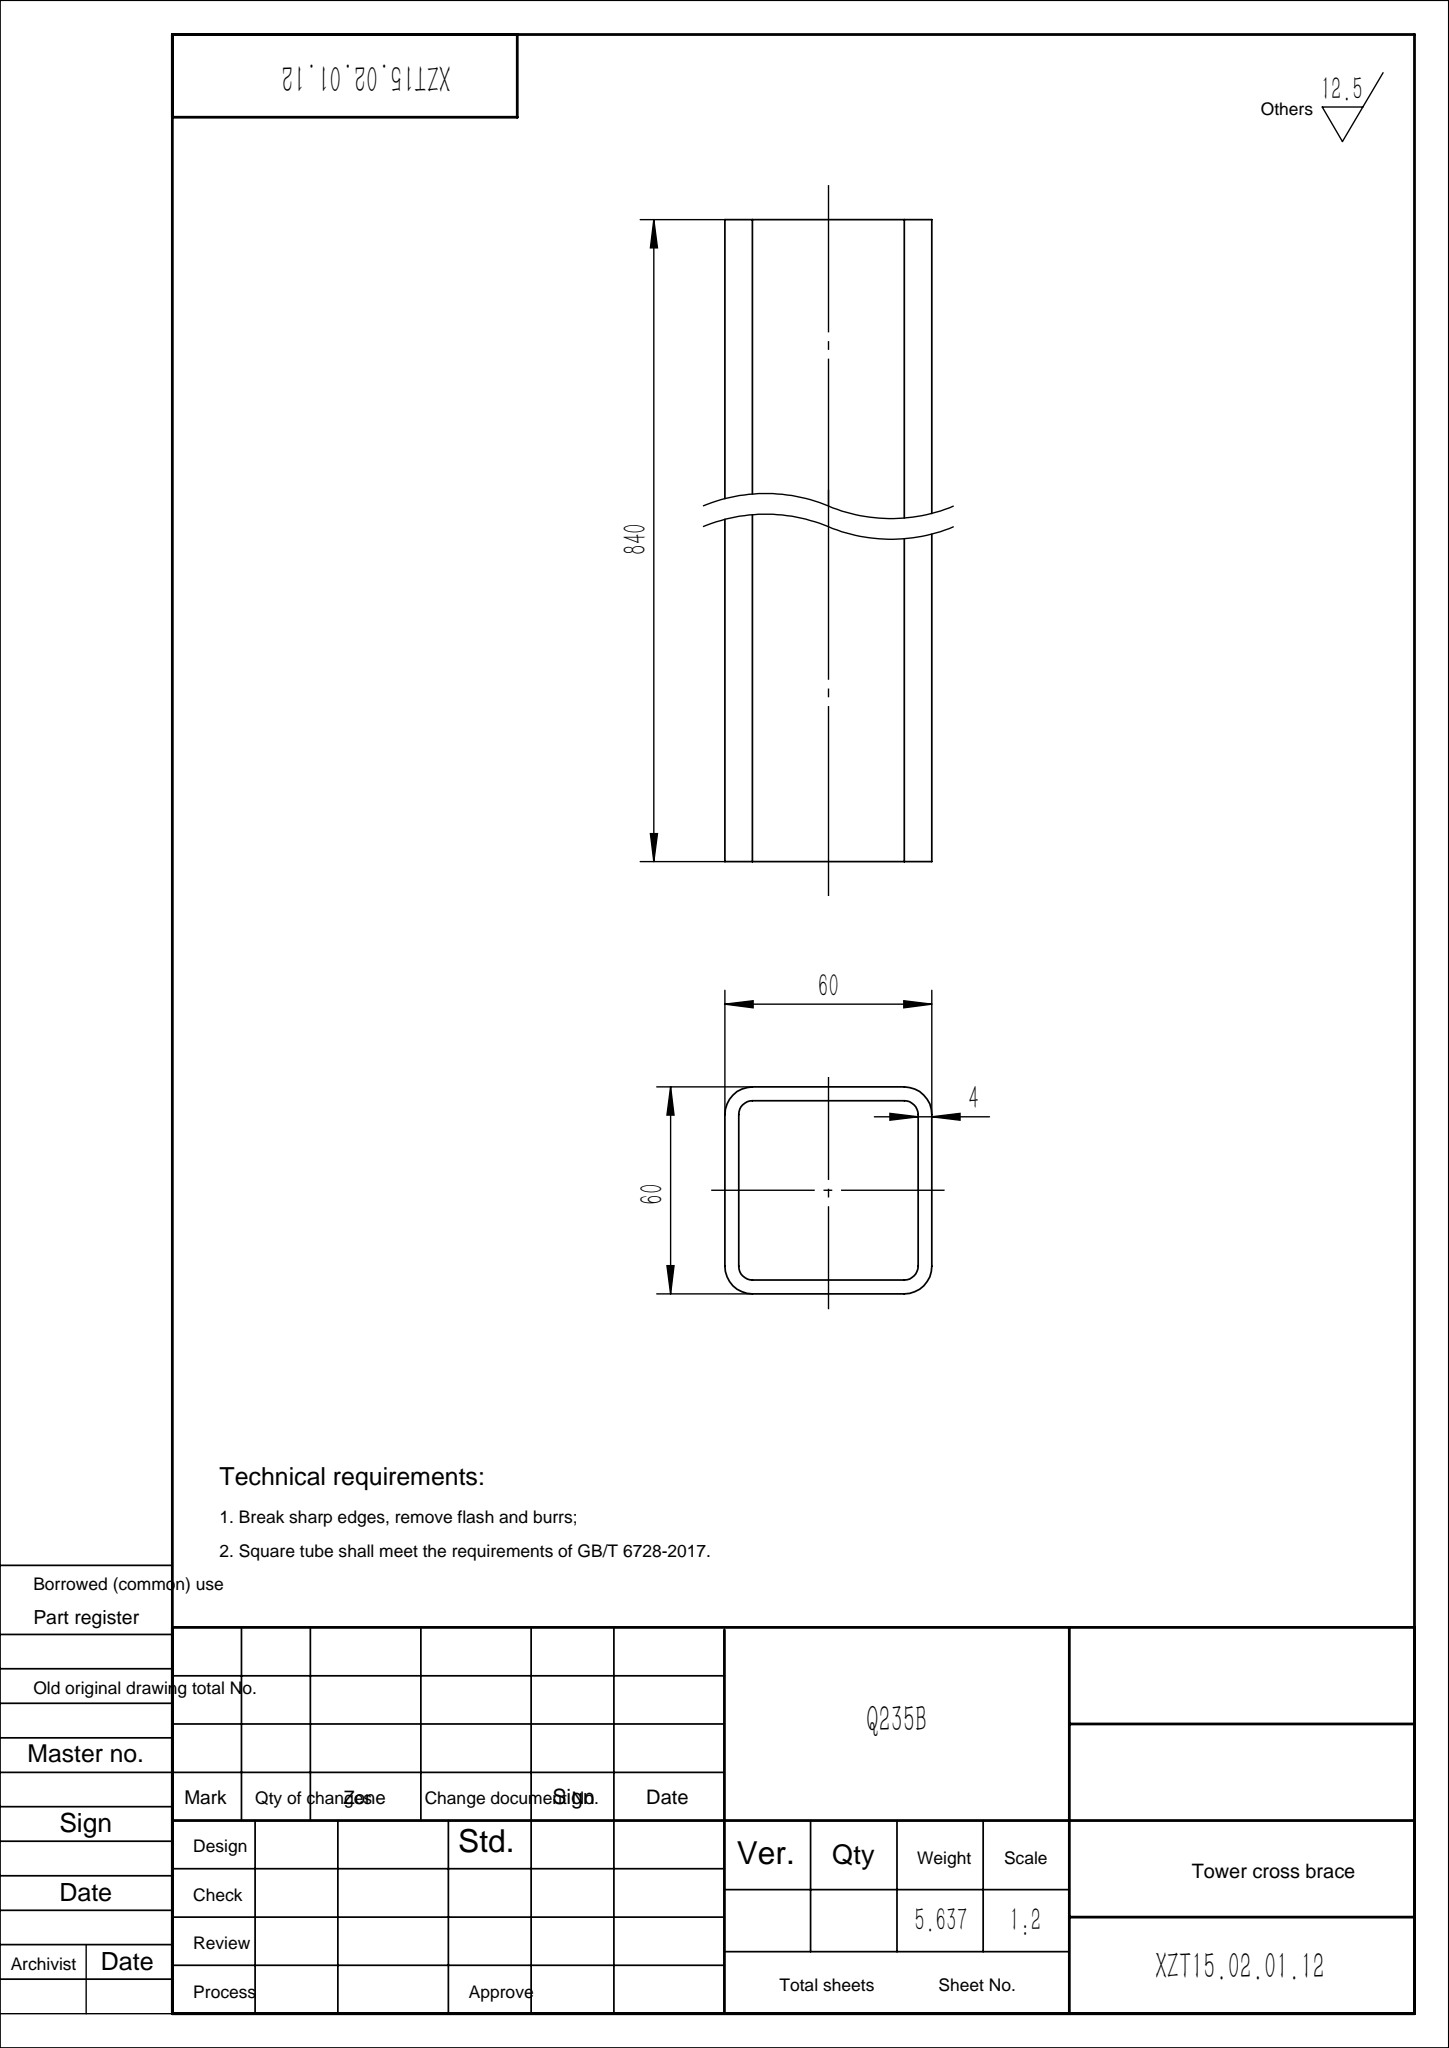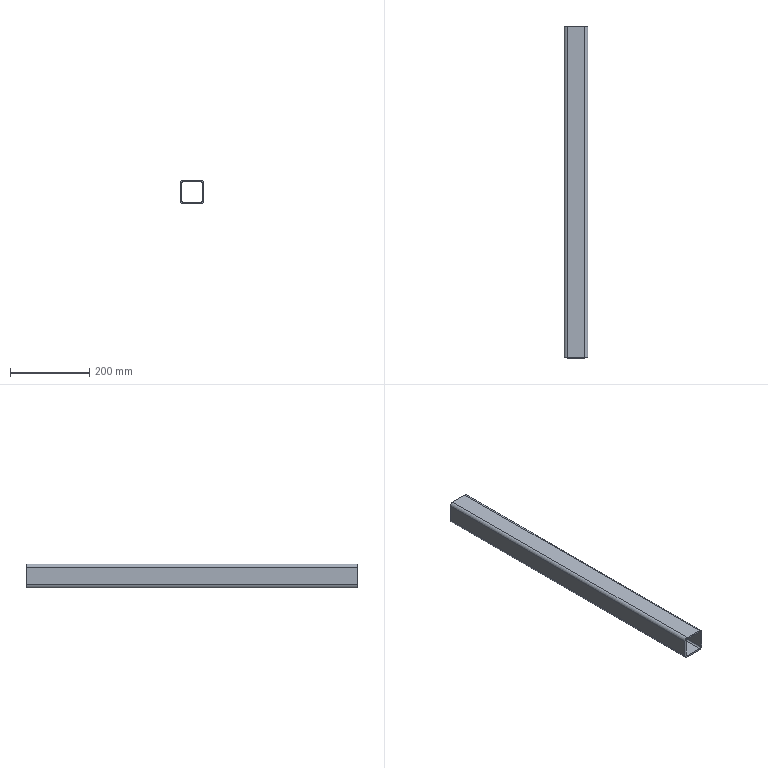Part | SolidWorks | features WeldMemberFeat 1, WeldmentFeature 1 | 1 solid | 18 faces | box 60 x 840 x 60 mm | volume 718029 mm3 | plane 10 | cylinder 8 | commonest cylinder face diameters 8 x4 16 x4
STEP:
#1=CARTESIAN_POINT('',(-30.,0.,22.));
#2=VERTEX_POINT('',#1);
#3=CARTESIAN_POINT('',(-22.,0.,30.));
#4=VERTEX_POINT('',#3);
#5=CARTESIAN_POINT('',(-22.,0.,22.));
#6=DIRECTION('',(0.,1.,0.));
#7=DIRECTION('',(0.,0.,1.));
#8=AXIS2_PLACEMENT_3D('',#5,#6,#7);
#9=CIRCLE('',#8,8.);
#10=EDGE_CURVE('',#2,#4,#9,.T.);
#11=ORIENTED_EDGE('',*,*,#10,.T.);
#12=CARTESIAN_POINT('',(-22.,840.,30.));
#13=VERTEX_POINT('',#12);
#14=CARTESIAN_POINT('',(-22.,840.,30.));
#15=DIRECTION('',(0.,-1.,0.));
#16=VECTOR('',#15,1000.);
#17=LINE('',#14,#16);
#18=EDGE_CURVE('',#13,#4,#17,.T.);
#19=ORIENTED_EDGE('',*,*,#18,.F.);
#20=CARTESIAN_POINT('',(-30.,840.,22.));
#21=VERTEX_POINT('',#20);
#22=CARTESIAN_POINT('',(-22.,840.,22.));
#23=DIRECTION('',(0.,1.,0.));
#24=DIRECTION('',(0.,0.,1.));
#25=AXIS2_PLACEMENT_3D('',#22,#23,#24);
#26=CIRCLE('',#25,8.);
#27=EDGE_CURVE('',#21,#13,#26,.T.);
#28=ORIENTED_EDGE('',*,*,#27,.F.);
#29=CARTESIAN_POINT('',(-30.,840.,22.));
#30=DIRECTION('',(0.,-1.,0.));
#31=VECTOR('',#30,1000.);
#32=LINE('',#29,#31);
#33=EDGE_CURVE('',#21,#2,#32,.T.);
#34=ORIENTED_EDGE('',*,*,#33,.T.);
#35=EDGE_LOOP('',(#11,#19,#28,#34));
#36=FACE_OUTER_BOUND('',#35,.T.);
#37=CARTESIAN_POINT('',(-22.,840.,22.));
#38=DIRECTION('',(0.,-1.,0.));
#39=DIRECTION('',(0.,0.,-1.));
#40=AXIS2_PLACEMENT_3D('',#37,#38,#39);
#41=CYLINDRICAL_SURFACE('',#40,8.);
#42=ADVANCED_FACE('',(#36),#41,.T.);
#43=CARTESIAN_POINT('',(22.,0.,30.));
#44=VERTEX_POINT('',#43);
#45=CARTESIAN_POINT('',(-22.,0.,30.));
#46=DIRECTION('',(1.,0.,0.));
#47=VECTOR('',#46,1000.);
#48=LINE('',#45,#47);
#49=EDGE_CURVE('',#4,#44,#48,.T.);
#50=ORIENTED_EDGE('',*,*,#49,.T.);
#51=CARTESIAN_POINT('',(22.,840.,30.));
#52=VERTEX_POINT('',#51);
#53=CARTESIAN_POINT('',(22.,840.,30.));
#54=DIRECTION('',(0.,-1.,0.));
#55=VECTOR('',#54,1000.);
#56=LINE('',#53,#55);
#57=EDGE_CURVE('',#52,#44,#56,.T.);
#58=ORIENTED_EDGE('',*,*,#57,.F.);
#59=CARTESIAN_POINT('',(-22.,840.,30.));
#60=DIRECTION('',(1.,0.,0.));
#61=VECTOR('',#60,1000.);
#62=LINE('',#59,#61);
#63=EDGE_CURVE('',#13,#52,#62,.T.);
#64=ORIENTED_EDGE('',*,*,#63,.F.);
#65=ORIENTED_EDGE('',*,*,#18,.T.);
#66=EDGE_LOOP('',(#50,#58,#64,#65));
#67=FACE_OUTER_BOUND('',#66,.T.);
#68=CARTESIAN_POINT('',(-22.,840.,30.));
#69=DIRECTION('',(0.,0.,-1.));
#70=DIRECTION('',(-1.,0.,0.));
#71=AXIS2_PLACEMENT_3D('',#68,#69,#70);
#72=PLANE('',#71);
#73=ADVANCED_FACE('',(#67),#72,.F.);
#74=CARTESIAN_POINT('',(30.,0.,22.));
#75=VERTEX_POINT('',#74);
#76=CARTESIAN_POINT('',(22.,0.,22.));
#77=DIRECTION('',(0.,1.,0.));
#78=DIRECTION('',(0.,0.,1.));
#79=AXIS2_PLACEMENT_3D('',#76,#77,#78);
#80=CIRCLE('',#79,8.);
#81=EDGE_CURVE('',#44,#75,#80,.T.);
#82=ORIENTED_EDGE('',*,*,#81,.T.);
#83=CARTESIAN_POINT('',(30.,840.,22.));
#84=VERTEX_POINT('',#83);
#85=CARTESIAN_POINT('',(30.,840.,22.));
#86=DIRECTION('',(0.,-1.,0.));
#87=VECTOR('',#86,1000.);
#88=LINE('',#85,#87);
#89=EDGE_CURVE('',#84,#75,#88,.T.);
#90=ORIENTED_EDGE('',*,*,#89,.F.);
#91=CARTESIAN_POINT('',(22.,840.,22.));
#92=DIRECTION('',(0.,1.,0.));
#93=DIRECTION('',(0.,0.,1.));
#94=AXIS2_PLACEMENT_3D('',#91,#92,#93);
#95=CIRCLE('',#94,8.);
#96=EDGE_CURVE('',#52,#84,#95,.T.);
#97=ORIENTED_EDGE('',*,*,#96,.F.);
#98=ORIENTED_EDGE('',*,*,#57,.T.);
#99=EDGE_LOOP('',(#82,#90,#97,#98));
#100=FACE_OUTER_BOUND('',#99,.T.);
#101=CARTESIAN_POINT('',(22.,840.,22.));
#102=DIRECTION('',(0.,-1.,0.));
#103=DIRECTION('',(0.,0.,-1.));
#104=AXIS2_PLACEMENT_3D('',#101,#102,#103);
#105=CYLINDRICAL_SURFACE('',#104,8.);
#106=ADVANCED_FACE('',(#100),#105,.T.);
#107=CARTESIAN_POINT('',(30.,0.,-22.));
#108=VERTEX_POINT('',#107);
#109=CARTESIAN_POINT('',(30.,0.,-22.));
#110=DIRECTION('',(0.,0.,-1.));
#111=VECTOR('',#110,1000.);
#112=LINE('',#109,#111);
#113=EDGE_CURVE('',#75,#108,#112,.T.);
#114=ORIENTED_EDGE('',*,*,#113,.T.);
#115=CARTESIAN_POINT('',(30.,840.,-22.));
#116=VERTEX_POINT('',#115);
#117=CARTESIAN_POINT('',(30.,840.,-22.));
#118=DIRECTION('',(0.,-1.,0.));
#119=VECTOR('',#118,1000.);
#120=LINE('',#117,#119);
#121=EDGE_CURVE('',#116,#108,#120,.T.);
#122=ORIENTED_EDGE('',*,*,#121,.F.);
#123=CARTESIAN_POINT('',(30.,840.,-22.));
#124=DIRECTION('',(0.,0.,-1.));
#125=VECTOR('',#124,1000.);
#126=LINE('',#123,#125);
#127=EDGE_CURVE('',#84,#116,#126,.T.);
#128=ORIENTED_EDGE('',*,*,#127,.F.);
#129=ORIENTED_EDGE('',*,*,#89,.T.);
#130=EDGE_LOOP('',(#114,#122,#128,#129));
#131=FACE_OUTER_BOUND('',#130,.T.);
#132=CARTESIAN_POINT('',(30.,840.,-22.));
#133=DIRECTION('',(-1.,0.,0.));
#134=DIRECTION('',(0.,0.,1.));
#135=AXIS2_PLACEMENT_3D('',#132,#133,#134);
#136=PLANE('',#135);
#137=ADVANCED_FACE('',(#131),#136,.F.);
#138=CARTESIAN_POINT('',(22.,0.,-30.));
#139=VERTEX_POINT('',#138);
#140=CARTESIAN_POINT('',(22.,0.,-22.));
#141=DIRECTION('',(0.,1.,0.));
#142=DIRECTION('',(0.,0.,1.));
#143=AXIS2_PLACEMENT_3D('',#140,#141,#142);
#144=CIRCLE('',#143,8.);
#145=EDGE_CURVE('',#108,#139,#144,.T.);
#146=ORIENTED_EDGE('',*,*,#145,.T.);
#147=CARTESIAN_POINT('',(22.,840.,-30.));
#148=VERTEX_POINT('',#147);
#149=CARTESIAN_POINT('',(22.,840.,-30.));
#150=DIRECTION('',(0.,-1.,0.));
#151=VECTOR('',#150,1000.);
#152=LINE('',#149,#151);
#153=EDGE_CURVE('',#148,#139,#152,.T.);
#154=ORIENTED_EDGE('',*,*,#153,.F.);
#155=CARTESIAN_POINT('',(22.,840.,-22.));
#156=DIRECTION('',(0.,1.,0.));
#157=DIRECTION('',(0.,0.,1.));
#158=AXIS2_PLACEMENT_3D('',#155,#156,#157);
#159=CIRCLE('',#158,8.);
#160=EDGE_CURVE('',#116,#148,#159,.T.);
#161=ORIENTED_EDGE('',*,*,#160,.F.);
#162=ORIENTED_EDGE('',*,*,#121,.T.);
#163=EDGE_LOOP('',(#146,#154,#161,#162));
#164=FACE_OUTER_BOUND('',#163,.T.);
#165=CARTESIAN_POINT('',(22.,840.,-22.));
#166=DIRECTION('',(0.,-1.,0.));
#167=DIRECTION('',(0.,0.,-1.));
#168=AXIS2_PLACEMENT_3D('',#165,#166,#167);
#169=CYLINDRICAL_SURFACE('',#168,8.);
#170=ADVANCED_FACE('',(#164),#169,.T.);
#171=CARTESIAN_POINT('',(-22.,0.,-30.));
#172=VERTEX_POINT('',#171);
#173=CARTESIAN_POINT('',(22.,0.,-30.));
#174=DIRECTION('',(-1.,0.,0.));
#175=VECTOR('',#174,1000.);
#176=LINE('',#173,#175);
#177=EDGE_CURVE('',#139,#172,#176,.T.);
#178=ORIENTED_EDGE('',*,*,#177,.T.);
#179=CARTESIAN_POINT('',(-22.,840.,-30.));
#180=VERTEX_POINT('',#179);
#181=CARTESIAN_POINT('',(-22.,840.,-30.));
#182=DIRECTION('',(0.,-1.,0.));
#183=VECTOR('',#182,1000.);
#184=LINE('',#181,#183);
#185=EDGE_CURVE('',#180,#172,#184,.T.);
#186=ORIENTED_EDGE('',*,*,#185,.F.);
#187=CARTESIAN_POINT('',(22.,840.,-30.));
#188=DIRECTION('',(-1.,0.,0.));
#189=VECTOR('',#188,1000.);
#190=LINE('',#187,#189);
#191=EDGE_CURVE('',#148,#180,#190,.T.);
#192=ORIENTED_EDGE('',*,*,#191,.F.);
#193=ORIENTED_EDGE('',*,*,#153,.T.);
#194=EDGE_LOOP('',(#178,#186,#192,#193));
#195=FACE_OUTER_BOUND('',#194,.T.);
#196=CARTESIAN_POINT('',(22.,840.,-30.));
#197=DIRECTION('',(0.,0.,1.));
#198=DIRECTION('',(1.,0.,0.));
#199=AXIS2_PLACEMENT_3D('',#196,#197,#198);
#200=PLANE('',#199);
#201=ADVANCED_FACE('',(#195),#200,.F.);
#202=CARTESIAN_POINT('',(-30.,0.,-22.));
#203=VERTEX_POINT('',#202);
#204=CARTESIAN_POINT('',(-22.,0.,-22.));
#205=DIRECTION('',(0.,1.,0.));
#206=DIRECTION('',(0.,0.,1.));
#207=AXIS2_PLACEMENT_3D('',#204,#205,#206);
#208=CIRCLE('',#207,8.);
#209=EDGE_CURVE('',#172,#203,#208,.T.);
#210=ORIENTED_EDGE('',*,*,#209,.T.);
#211=CARTESIAN_POINT('',(-30.,840.,-22.));
#212=VERTEX_POINT('',#211);
#213=CARTESIAN_POINT('',(-30.,840.,-22.));
#214=DIRECTION('',(0.,-1.,0.));
#215=VECTOR('',#214,1000.);
#216=LINE('',#213,#215);
#217=EDGE_CURVE('',#212,#203,#216,.T.);
#218=ORIENTED_EDGE('',*,*,#217,.F.);
#219=CARTESIAN_POINT('',(-22.,840.,-22.));
#220=DIRECTION('',(0.,1.,0.));
#221=DIRECTION('',(0.,0.,1.));
#222=AXIS2_PLACEMENT_3D('',#219,#220,#221);
#223=CIRCLE('',#222,8.);
#224=EDGE_CURVE('',#180,#212,#223,.T.);
#225=ORIENTED_EDGE('',*,*,#224,.F.);
#226=ORIENTED_EDGE('',*,*,#185,.T.);
#227=EDGE_LOOP('',(#210,#218,#225,#226));
#228=FACE_OUTER_BOUND('',#227,.T.);
#229=CARTESIAN_POINT('',(-22.,840.,-22.));
#230=DIRECTION('',(0.,-1.,0.));
#231=DIRECTION('',(0.,0.,-1.));
#232=AXIS2_PLACEMENT_3D('',#229,#230,#231);
#233=CYLINDRICAL_SURFACE('',#232,8.);
#234=ADVANCED_FACE('',(#228),#233,.T.);
#235=CARTESIAN_POINT('',(22.,0.,26.));
#236=VERTEX_POINT('',#235);
#237=CARTESIAN_POINT('',(26.,0.,22.));
#238=VERTEX_POINT('',#237);
#239=CARTESIAN_POINT('',(22.,0.,22.));
#240=DIRECTION('',(0.,1.,0.));
#241=DIRECTION('',(0.,0.,1.));
#242=AXIS2_PLACEMENT_3D('',#239,#240,#241);
#243=CIRCLE('',#242,4.);
#244=EDGE_CURVE('',#236,#238,#243,.T.);
#245=ORIENTED_EDGE('',*,*,#244,.F.);
#246=CARTESIAN_POINT('',(22.,840.,26.));
#247=VERTEX_POINT('',#246);
#248=CARTESIAN_POINT('',(22.,840.,26.));
#249=DIRECTION('',(0.,-1.,0.));
#250=VECTOR('',#249,1000.);
#251=LINE('',#248,#250);
#252=EDGE_CURVE('',#247,#236,#251,.T.);
#253=ORIENTED_EDGE('',*,*,#252,.F.);
#254=CARTESIAN_POINT('',(26.,840.,22.));
#255=VERTEX_POINT('',#254);
#256=CARTESIAN_POINT('',(22.,840.,22.));
#257=DIRECTION('',(0.,1.,0.));
#258=DIRECTION('',(0.,0.,1.));
#259=AXIS2_PLACEMENT_3D('',#256,#257,#258);
#260=CIRCLE('',#259,4.);
#261=EDGE_CURVE('',#247,#255,#260,.T.);
#262=ORIENTED_EDGE('',*,*,#261,.T.);
#263=CARTESIAN_POINT('',(26.,840.,22.));
#264=DIRECTION('',(0.,-1.,0.));
#265=VECTOR('',#264,1000.);
#266=LINE('',#263,#265);
#267=EDGE_CURVE('',#255,#238,#266,.T.);
#268=ORIENTED_EDGE('',*,*,#267,.T.);
#269=EDGE_LOOP('',(#245,#253,#262,#268));
#270=FACE_OUTER_BOUND('',#269,.T.);
#271=CARTESIAN_POINT('',(22.,840.,22.));
#272=DIRECTION('',(0.,-1.,0.));
#273=DIRECTION('',(0.,0.,-1.));
#274=AXIS2_PLACEMENT_3D('',#271,#272,#273);
#275=CYLINDRICAL_SURFACE('',#274,4.);
#276=ADVANCED_FACE('',(#270),#275,.F.);
#277=CARTESIAN_POINT('',(-22.,0.,26.));
#278=VERTEX_POINT('',#277);
#279=CARTESIAN_POINT('',(-22.,0.,26.));
#280=DIRECTION('',(1.,0.,0.));
#281=VECTOR('',#280,1000.);
#282=LINE('',#279,#281);
#283=EDGE_CURVE('',#278,#236,#282,.T.);
#284=ORIENTED_EDGE('',*,*,#283,.F.);
#285=CARTESIAN_POINT('',(-22.,840.,26.));
#286=VERTEX_POINT('',#285);
#287=CARTESIAN_POINT('',(-22.,840.,26.));
#288=DIRECTION('',(0.,-1.,0.));
#289=VECTOR('',#288,1000.);
#290=LINE('',#287,#289);
#291=EDGE_CURVE('',#286,#278,#290,.T.);
#292=ORIENTED_EDGE('',*,*,#291,.F.);
#293=CARTESIAN_POINT('',(-22.,840.,26.));
#294=DIRECTION('',(1.,0.,0.));
#295=VECTOR('',#294,1000.);
#296=LINE('',#293,#295);
#297=EDGE_CURVE('',#286,#247,#296,.T.);
#298=ORIENTED_EDGE('',*,*,#297,.T.);
#299=ORIENTED_EDGE('',*,*,#252,.T.);
#300=EDGE_LOOP('',(#284,#292,#298,#299));
#301=FACE_OUTER_BOUND('',#300,.T.);
#302=CARTESIAN_POINT('',(-22.,840.,26.));
#303=DIRECTION('',(0.,0.,-1.));
#304=DIRECTION('',(-1.,0.,0.));
#305=AXIS2_PLACEMENT_3D('',#302,#303,#304);
#306=PLANE('',#305);
#307=ADVANCED_FACE('',(#301),#306,.T.);
#308=CARTESIAN_POINT('',(-26.,0.,22.));
#309=VERTEX_POINT('',#308);
#310=CARTESIAN_POINT('',(-22.,0.,22.));
#311=DIRECTION('',(0.,1.,0.));
#312=DIRECTION('',(0.,0.,1.));
#313=AXIS2_PLACEMENT_3D('',#310,#311,#312);
#314=CIRCLE('',#313,4.);
#315=EDGE_CURVE('',#309,#278,#314,.T.);
#316=ORIENTED_EDGE('',*,*,#315,.F.);
#317=CARTESIAN_POINT('',(-26.,840.,22.));
#318=VERTEX_POINT('',#317);
#319=CARTESIAN_POINT('',(-26.,840.,22.));
#320=DIRECTION('',(0.,-1.,0.));
#321=VECTOR('',#320,1000.);
#322=LINE('',#319,#321);
#323=EDGE_CURVE('',#318,#309,#322,.T.);
#324=ORIENTED_EDGE('',*,*,#323,.F.);
#325=CARTESIAN_POINT('',(-22.,840.,22.));
#326=DIRECTION('',(0.,1.,0.));
#327=DIRECTION('',(0.,0.,1.));
#328=AXIS2_PLACEMENT_3D('',#325,#326,#327);
#329=CIRCLE('',#328,4.);
#330=EDGE_CURVE('',#318,#286,#329,.T.);
#331=ORIENTED_EDGE('',*,*,#330,.T.);
#332=ORIENTED_EDGE('',*,*,#291,.T.);
#333=EDGE_LOOP('',(#316,#324,#331,#332));
#334=FACE_OUTER_BOUND('',#333,.T.);
#335=CARTESIAN_POINT('',(-22.,840.,22.));
#336=DIRECTION('',(0.,-1.,0.));
#337=DIRECTION('',(0.,0.,-1.));
#338=AXIS2_PLACEMENT_3D('',#335,#336,#337);
#339=CYLINDRICAL_SURFACE('',#338,4.);
#340=ADVANCED_FACE('',(#334),#339,.F.);
#341=CARTESIAN_POINT('',(-26.,0.,-22.));
#342=VERTEX_POINT('',#341);
#343=CARTESIAN_POINT('',(-26.,0.,22.));
#344=DIRECTION('',(0.,0.,1.));
#345=VECTOR('',#344,1000.);
#346=LINE('',#343,#345);
#347=EDGE_CURVE('',#342,#309,#346,.T.);
#348=ORIENTED_EDGE('',*,*,#347,.F.);
#349=CARTESIAN_POINT('',(-26.,840.,-22.));
#350=VERTEX_POINT('',#349);
#351=CARTESIAN_POINT('',(-26.,840.,-22.));
#352=DIRECTION('',(0.,-1.,0.));
#353=VECTOR('',#352,1000.);
#354=LINE('',#351,#353);
#355=EDGE_CURVE('',#350,#342,#354,.T.);
#356=ORIENTED_EDGE('',*,*,#355,.F.);
#357=CARTESIAN_POINT('',(-26.,840.,22.));
#358=DIRECTION('',(0.,0.,1.));
#359=VECTOR('',#358,1000.);
#360=LINE('',#357,#359);
#361=EDGE_CURVE('',#350,#318,#360,.T.);
#362=ORIENTED_EDGE('',*,*,#361,.T.);
#363=ORIENTED_EDGE('',*,*,#323,.T.);
#364=EDGE_LOOP('',(#348,#356,#362,#363));
#365=FACE_OUTER_BOUND('',#364,.T.);
#366=CARTESIAN_POINT('',(-26.,840.,22.));
#367=DIRECTION('',(1.,0.,0.));
#368=DIRECTION('',(0.,0.,-1.));
#369=AXIS2_PLACEMENT_3D('',#366,#367,#368);
#370=PLANE('',#369);
#371=ADVANCED_FACE('',(#365),#370,.T.);
#372=CARTESIAN_POINT('',(-22.,0.,-26.));
#373=VERTEX_POINT('',#372);
#374=CARTESIAN_POINT('',(-22.,0.,-22.));
#375=DIRECTION('',(0.,1.,0.));
#376=DIRECTION('',(0.,0.,1.));
#377=AXIS2_PLACEMENT_3D('',#374,#375,#376);
#378=CIRCLE('',#377,4.);
#379=EDGE_CURVE('',#373,#342,#378,.T.);
#380=ORIENTED_EDGE('',*,*,#379,.F.);
#381=CARTESIAN_POINT('',(-22.,840.,-26.));
#382=VERTEX_POINT('',#381);
#383=CARTESIAN_POINT('',(-22.,840.,-26.));
#384=DIRECTION('',(0.,-1.,0.));
#385=VECTOR('',#384,1000.);
#386=LINE('',#383,#385);
#387=EDGE_CURVE('',#382,#373,#386,.T.);
#388=ORIENTED_EDGE('',*,*,#387,.F.);
#389=CARTESIAN_POINT('',(-22.,840.,-22.));
#390=DIRECTION('',(0.,1.,0.));
#391=DIRECTION('',(0.,0.,1.));
#392=AXIS2_PLACEMENT_3D('',#389,#390,#391);
#393=CIRCLE('',#392,4.);
#394=EDGE_CURVE('',#382,#350,#393,.T.);
#395=ORIENTED_EDGE('',*,*,#394,.T.);
#396=ORIENTED_EDGE('',*,*,#355,.T.);
#397=EDGE_LOOP('',(#380,#388,#395,#396));
#398=FACE_OUTER_BOUND('',#397,.T.);
#399=CARTESIAN_POINT('',(-22.,840.,-22.));
#400=DIRECTION('',(0.,-1.,0.));
#401=DIRECTION('',(0.,0.,-1.));
#402=AXIS2_PLACEMENT_3D('',#399,#400,#401);
#403=CYLINDRICAL_SURFACE('',#402,4.);
#404=ADVANCED_FACE('',(#398),#403,.F.);
#405=CARTESIAN_POINT('',(22.,0.,-26.));
#406=VERTEX_POINT('',#405);
#407=CARTESIAN_POINT('',(22.,0.,-26.));
#408=DIRECTION('',(-1.,0.,0.));
#409=VECTOR('',#408,1000.);
#410=LINE('',#407,#409);
#411=EDGE_CURVE('',#406,#373,#410,.T.);
#412=ORIENTED_EDGE('',*,*,#411,.F.);
#413=CARTESIAN_POINT('',(22.,840.,-26.));
#414=VERTEX_POINT('',#413);
#415=CARTESIAN_POINT('',(22.,840.,-26.));
#416=DIRECTION('',(0.,-1.,0.));
#417=VECTOR('',#416,1000.);
#418=LINE('',#415,#417);
#419=EDGE_CURVE('',#414,#406,#418,.T.);
#420=ORIENTED_EDGE('',*,*,#419,.F.);
#421=CARTESIAN_POINT('',(22.,840.,-26.));
#422=DIRECTION('',(-1.,0.,0.));
#423=VECTOR('',#422,1000.);
#424=LINE('',#421,#423);
#425=EDGE_CURVE('',#414,#382,#424,.T.);
#426=ORIENTED_EDGE('',*,*,#425,.T.);
#427=ORIENTED_EDGE('',*,*,#387,.T.);
#428=EDGE_LOOP('',(#412,#420,#426,#427));
#429=FACE_OUTER_BOUND('',#428,.T.);
#430=CARTESIAN_POINT('',(22.,840.,-26.));
#431=DIRECTION('',(0.,0.,1.));
#432=DIRECTION('',(1.,0.,0.));
#433=AXIS2_PLACEMENT_3D('',#430,#431,#432);
#434=PLANE('',#433);
#435=ADVANCED_FACE('',(#429),#434,.T.);
#436=CARTESIAN_POINT('',(26.,0.,-22.));
#437=VERTEX_POINT('',#436);
#438=CARTESIAN_POINT('',(22.,0.,-22.));
#439=DIRECTION('',(0.,1.,0.));
#440=DIRECTION('',(0.,0.,1.));
#441=AXIS2_PLACEMENT_3D('',#438,#439,#440);
#442=CIRCLE('',#441,4.);
#443=EDGE_CURVE('',#437,#406,#442,.T.);
#444=ORIENTED_EDGE('',*,*,#443,.F.);
#445=CARTESIAN_POINT('',(26.,840.,-22.));
#446=VERTEX_POINT('',#445);
#447=CARTESIAN_POINT('',(26.,840.,-22.));
#448=DIRECTION('',(0.,-1.,0.));
#449=VECTOR('',#448,1000.);
#450=LINE('',#447,#449);
#451=EDGE_CURVE('',#446,#437,#450,.T.);
#452=ORIENTED_EDGE('',*,*,#451,.F.);
#453=CARTESIAN_POINT('',(22.,840.,-22.));
#454=DIRECTION('',(0.,1.,0.));
#455=DIRECTION('',(0.,0.,1.));
#456=AXIS2_PLACEMENT_3D('',#453,#454,#455);
#457=CIRCLE('',#456,4.);
#458=EDGE_CURVE('',#446,#414,#457,.T.);
#459=ORIENTED_EDGE('',*,*,#458,.T.);
#460=ORIENTED_EDGE('',*,*,#419,.T.);
#461=EDGE_LOOP('',(#444,#452,#459,#460));
#462=FACE_OUTER_BOUND('',#461,.T.);
#463=CARTESIAN_POINT('',(22.,840.,-22.));
#464=DIRECTION('',(0.,-1.,0.));
#465=DIRECTION('',(0.,0.,-1.));
#466=AXIS2_PLACEMENT_3D('',#463,#464,#465);
#467=CYLINDRICAL_SURFACE('',#466,4.);
#468=ADVANCED_FACE('',(#462),#467,.F.);
#469=CARTESIAN_POINT('',(26.,0.,-22.));
#470=DIRECTION('',(0.,0.,-1.));
#471=VECTOR('',#470,1000.);
#472=LINE('',#469,#471);
#473=EDGE_CURVE('',#238,#437,#472,.T.);
#474=ORIENTED_EDGE('',*,*,#473,.F.);
#475=ORIENTED_EDGE('',*,*,#267,.F.);
#476=CARTESIAN_POINT('',(26.,840.,-22.));
#477=DIRECTION('',(0.,0.,-1.));
#478=VECTOR('',#477,1000.);
#479=LINE('',#476,#478);
#480=EDGE_CURVE('',#255,#446,#479,.T.);
#481=ORIENTED_EDGE('',*,*,#480,.T.);
#482=ORIENTED_EDGE('',*,*,#451,.T.);
#483=EDGE_LOOP('',(#474,#475,#481,#482));
#484=FACE_OUTER_BOUND('',#483,.T.);
#485=CARTESIAN_POINT('',(26.,840.,-22.));
#486=DIRECTION('',(-1.,0.,0.));
#487=DIRECTION('',(0.,0.,1.));
#488=AXIS2_PLACEMENT_3D('',#485,#486,#487);
#489=PLANE('',#488);
#490=ADVANCED_FACE('',(#484),#489,.T.);
#491=CARTESIAN_POINT('',(-30.,0.,22.));
#492=DIRECTION('',(0.,0.,1.));
#493=VECTOR('',#492,1000.);
#494=LINE('',#491,#493);
#495=EDGE_CURVE('',#203,#2,#494,.T.);
#496=ORIENTED_EDGE('',*,*,#495,.T.);
#497=ORIENTED_EDGE('',*,*,#33,.F.);
#498=CARTESIAN_POINT('',(-30.,840.,22.));
#499=DIRECTION('',(0.,0.,1.));
#500=VECTOR('',#499,1000.);
#501=LINE('',#498,#500);
#502=EDGE_CURVE('',#212,#21,#501,.T.);
#503=ORIENTED_EDGE('',*,*,#502,.F.);
#504=ORIENTED_EDGE('',*,*,#217,.T.);
#505=EDGE_LOOP('',(#496,#497,#503,#504));
#506=FACE_OUTER_BOUND('',#505,.T.);
#507=CARTESIAN_POINT('',(-30.,840.,22.));
#508=DIRECTION('',(1.,0.,0.));
#509=DIRECTION('',(0.,0.,-1.));
#510=AXIS2_PLACEMENT_3D('',#507,#508,#509);
#511=PLANE('',#510);
#512=ADVANCED_FACE('',(#506),#511,.F.);
#513=ORIENTED_EDGE('',*,*,#261,.F.);
#514=ORIENTED_EDGE('',*,*,#297,.F.);
#515=ORIENTED_EDGE('',*,*,#330,.F.);
#516=ORIENTED_EDGE('',*,*,#361,.F.);
#517=ORIENTED_EDGE('',*,*,#394,.F.);
#518=ORIENTED_EDGE('',*,*,#425,.F.);
#519=ORIENTED_EDGE('',*,*,#458,.F.);
#520=ORIENTED_EDGE('',*,*,#480,.F.);
#521=EDGE_LOOP('',(#513,#514,#515,#516,#517,#518,#519,#520));
#522=FACE_BOUND('',#521,.T.);
#523=ORIENTED_EDGE('',*,*,#27,.T.);
#524=ORIENTED_EDGE('',*,*,#63,.T.);
#525=ORIENTED_EDGE('',*,*,#96,.T.);
#526=ORIENTED_EDGE('',*,*,#127,.T.);
#527=ORIENTED_EDGE('',*,*,#160,.T.);
#528=ORIENTED_EDGE('',*,*,#191,.T.);
#529=ORIENTED_EDGE('',*,*,#224,.T.);
#530=ORIENTED_EDGE('',*,*,#502,.T.);
#531=EDGE_LOOP('',(#523,#524,#525,#526,#527,#528,#529,#530));
#532=FACE_OUTER_BOUND('',#531,.T.);
#533=CARTESIAN_POINT('',(-22.,840.,22.));
#534=DIRECTION('',(0.,1.,0.));
#535=DIRECTION('',(0.,0.,1.));
#536=AXIS2_PLACEMENT_3D('',#533,#534,#535);
#537=PLANE('',#536);
#538=ADVANCED_FACE('',(#522,#532),#537,.T.);
#539=ORIENTED_EDGE('',*,*,#244,.T.);
#540=ORIENTED_EDGE('',*,*,#473,.T.);
#541=ORIENTED_EDGE('',*,*,#443,.T.);
#542=ORIENTED_EDGE('',*,*,#411,.T.);
#543=ORIENTED_EDGE('',*,*,#379,.T.);
#544=ORIENTED_EDGE('',*,*,#347,.T.);
#545=ORIENTED_EDGE('',*,*,#315,.T.);
#546=ORIENTED_EDGE('',*,*,#283,.T.);
#547=EDGE_LOOP('',(#539,#540,#541,#542,#543,#544,#545,#546));
#548=FACE_BOUND('',#547,.T.);
#549=ORIENTED_EDGE('',*,*,#10,.F.);
#550=ORIENTED_EDGE('',*,*,#495,.F.);
#551=ORIENTED_EDGE('',*,*,#209,.F.);
#552=ORIENTED_EDGE('',*,*,#177,.F.);
#553=ORIENTED_EDGE('',*,*,#145,.F.);
#554=ORIENTED_EDGE('',*,*,#113,.F.);
#555=ORIENTED_EDGE('',*,*,#81,.F.);
#556=ORIENTED_EDGE('',*,*,#49,.F.);
#557=EDGE_LOOP('',(#549,#550,#551,#552,#553,#554,#555,#556));
#558=FACE_OUTER_BOUND('',#557,.T.);
#559=CARTESIAN_POINT('',(-22.,0.,22.));
#560=DIRECTION('',(0.,1.,0.));
#561=DIRECTION('',(0.,0.,1.));
#562=AXIS2_PLACEMENT_3D('',#559,#560,#561);
#563=PLANE('',#562);
#564=ADVANCED_FACE('',(#548,#558),#563,.F.);
#565=CLOSED_SHELL('',(#42,#73,#106,#137,#170,#201,#234,#276,#307,#340,#371,#404,#435,#468,#490,#512,#538,#564));
#566=MANIFOLD_SOLID_BREP('',#565);
#567=CARTESIAN_POINT('',(0.,0.,0.));
#568=DIRECTION('',(0.,0.,1.));
#569=DIRECTION('',(1.,0.,0.));
#570=AXIS2_PLACEMENT_3D('',#567,#568,#569);
#571=(LENGTH_UNIT()NAMED_UNIT(*)SI_UNIT(.MILLI.,.METRE.));
#572=UNCERTAINTY_MEASURE_WITH_UNIT(LENGTH_MEASURE(0.00001),#571,'','');
#573=(NAMED_UNIT(*)PLANE_ANGLE_UNIT()SI_UNIT($,.RADIAN.));
#574=(NAMED_UNIT(*)SI_UNIT($,.STERADIAN.)SOLID_ANGLE_UNIT());
#575=(GEOMETRIC_REPRESENTATION_CONTEXT(3)GLOBAL_UNCERTAINTY_ASSIGNED_CONTEXT((#572))GLOBAL_UNIT_ASSIGNED_CONTEXT((#571,#573,#574))REPRESENTATION_CONTEXT('',''));
#576=ADVANCED_BREP_SHAPE_REPRESENTATION('',(#566,#570),#575);